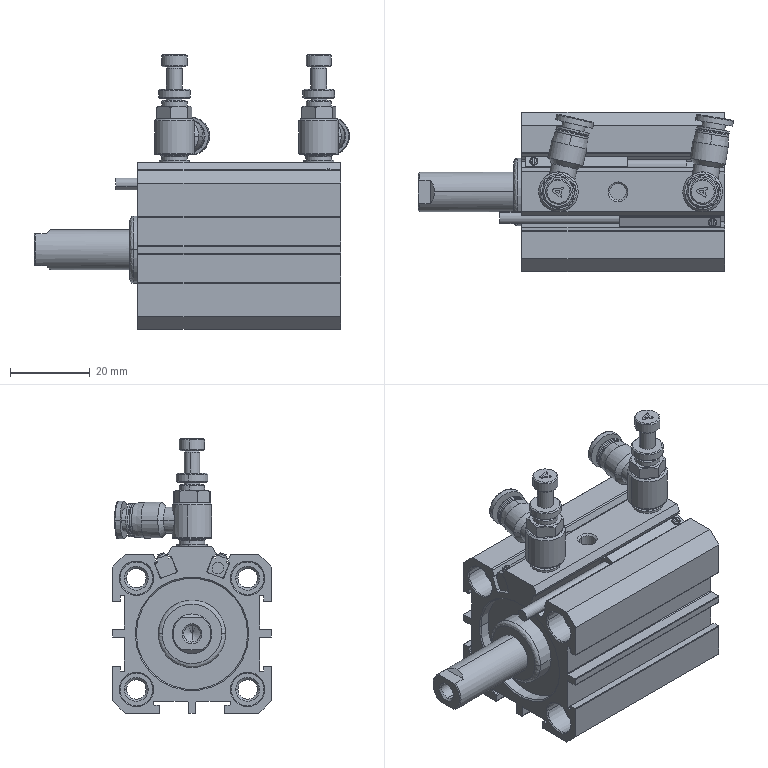Part | SolidWorks | features BaseBody 6, MoveFace 2 | 6 solids | 559 faces | box 79.253 x 40 x 69.1 mm | volume 68405 mm3 | plane 216 | cylinder 199 | cone 122 | spline 22 | commonest cylinder face diameters 0.4 x50 8.2 x16 4 x12 4.917 x8 6.4 x8 8.4 x8